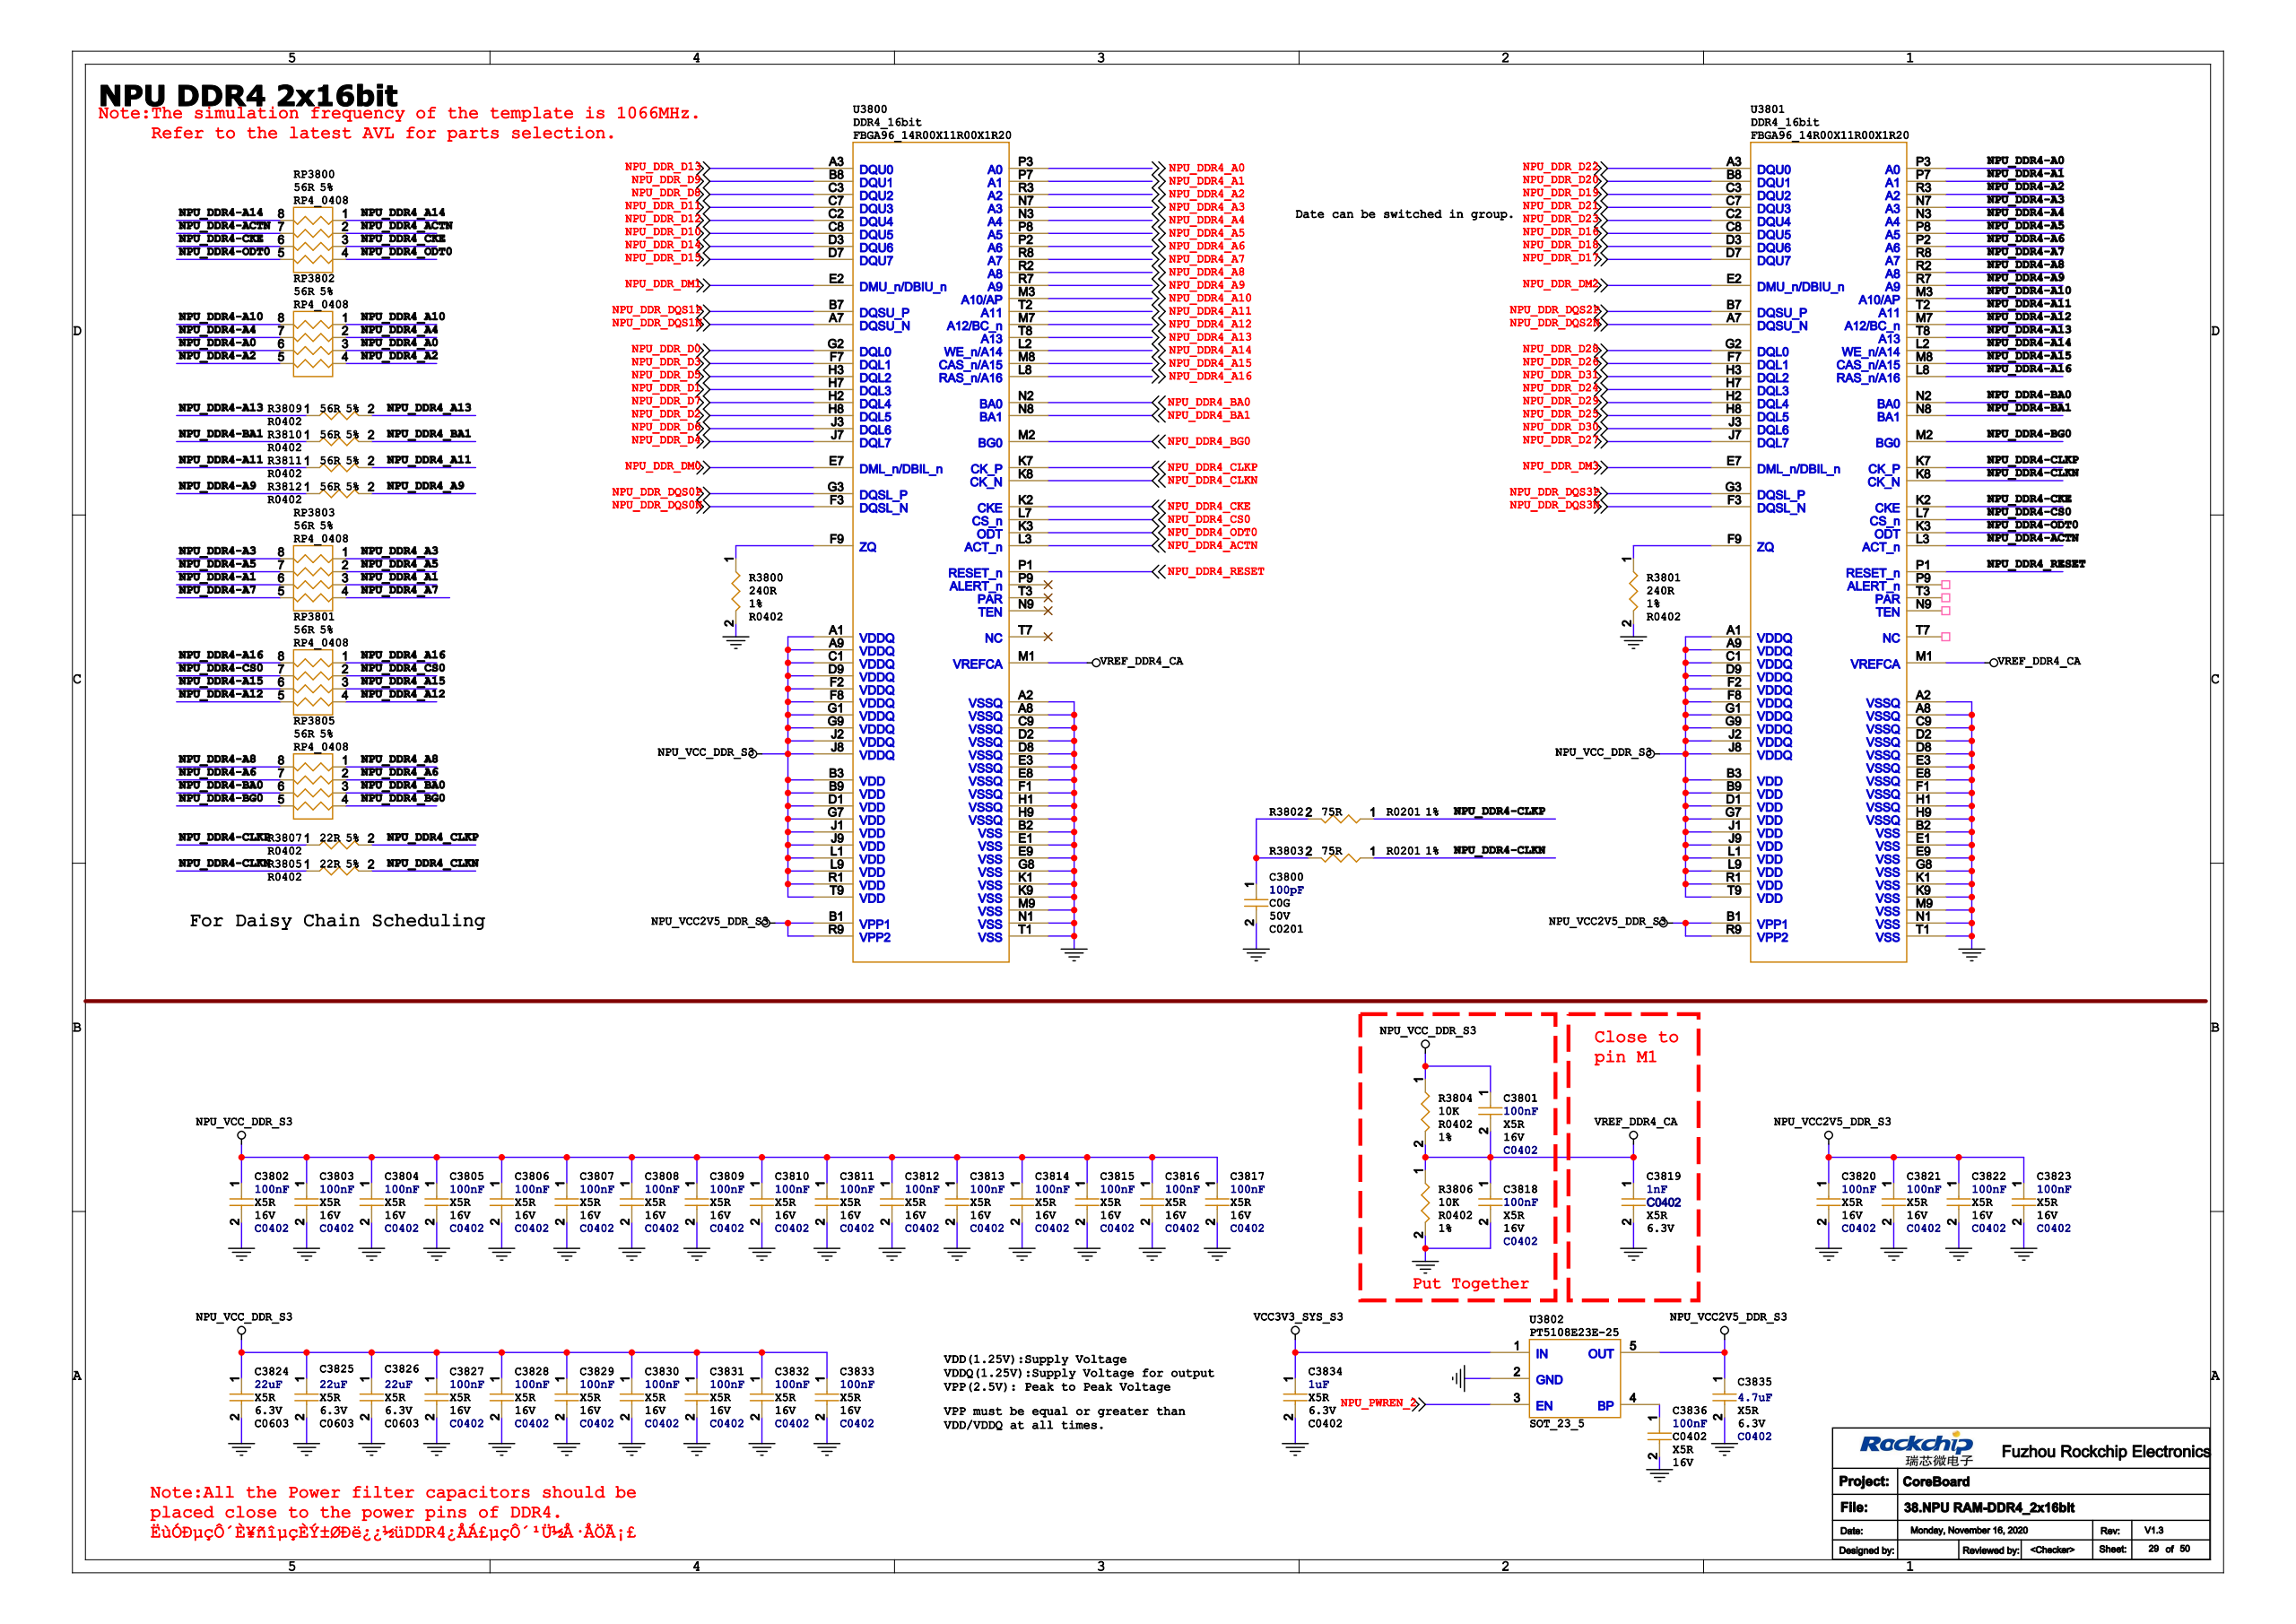Circuit board | Cadence Allegro | 749 parts | 717 nets | one sheet of the schematic
Parts on this sheet (reference | value | footprint):
C3800 | 100pF | C0201
C3801 | 100nF | C0402
C3802 | 100nF | C0402
C3803 | 100nF | C0402
C3804 | 100nF | C0402
C3805 | 100nF | C0402
C3806 | 100nF | C0402
C3807 | 100nF | C0402
C3808 | 100nF | C0402
C3809 | 100nF | C0402
C3810 | 100nF | C0402
C3811 | 100nF | C0402
C3812 | 100nF | C0402
C3813 | 100nF | C0402
C3814 | 100nF | C0402
C3815 | 100nF | C0402
C3816 | 100nF | C0402
C3817 | 100nF | C0402
C3818 | 100nF | C0402
C3819 | 1nF | C0402
C3820 | 100nF | C0402
C3821 | 100nF | C0402
C3822 | 100nF | C0402
C3823 | 100nF | C0402
C3824 | 22uF | C0603
C3825 | 22uF | C0603
C3826 | 22uF | C0603
C3827 | 100nF | C0402
C3828 | 100nF | C0402
C3829 | 100nF | C0402
C3830 | 100nF | C0402
C3831 | 100nF | C0402
C3832 | 100nF | C0402
C3833 | 100nF | C0402
C3834 | 1uF | C0402
C3835 | 4.7uF | C0402
C3836 | 100nF | C0402
R3800 | 240R | R0402
R3801 | 240R | R0402
R3804 | 10K | R0402
R3805 | 22R | R0402
R3806 | 10K | R0402
R3807 | 22R | R0402
R3809 | 56R | R0402
R3810 | 56R | R0402
R3811 | 56R | R0402
R3812 | 56R | R0402
RP3800 | 56R | RP4_0408
RP3801 | 56R | RP4_0408
RP3802 | 56R | RP4_0408
RP3803 | 56R | RP4_0408
RP3805 | 56R | RP4_0408
U3800 | DDR4_16bit | FBGA96_14R00X11R00X1R20
U3801 | DDR4_16bit | FBGA96_14R00X11R00X1R20
U3802 | PT5108E23E-25 | SOT_23_5
Nets of these parts (net: part-pin ...):
GND: C3800-2 C3802-2 C3803-2 C3804-2 C3805-2 C3806-2 C3807-2 C3808-2 C3809-2 C3810-2 C3811-2 C3812-2 C3813-2 C3814-2 C3815-2 C3816-2 C3817-2 C3818-2 C3819-2 C3820-2 C3821-2 C3822-2 C3823-2 C3824-2 C3825-2 C3826-2 C3827-2 C3828-2 C3829-2 C3830-2 C3831-2 C3832-2 C3833-2 C3834-2 C3835-2 C3836-2 R3800-2 R3801-2 R3806-2 U3802-2 U3800-A2 U3800-A8 U3800-B2 U3800-C9 U3800-D2 U3800-D8 U3800-E1 U3800-E3 U3800-E8 U3800-E9 U3800-F1 U3800-G8 U3800-H1 U3800-H9 U3800-K1 U3800-K9 U3800-M9 U3800-N1 U3800-T1 U3801-A2 U3801-A8 U3801-B2 U3801-C9 U3801-D2 U3801-D8 U3801-E1 U3801-E3 U3801-E8 U3801-E9 U3801-F1 U3801-G8 U3801-H1 U3801-H9 U3801-K1 U3801-K9 U3801-M9 U3801-N1 U3801-T1
VCC3V3_SYS_S3: C3834-1 U3802-1
NPU_VCC_DDR_S3: C3801-1 C3802-1 C3803-1 C3804-1 C3805-1 C3806-1 C3807-1 C3808-1 C3809-1 C3810-1 C3811-1 C3812-1 C3813-1 C3814-1 C3815-1 C3816-1 C3817-1 C3824-1 C3825-1 C3826-1 C3827-1 C3828-1 C3829-1 C3830-1 C3831-1 C3832-1 C3833-1 R3804-1 U3800-A1 U3800-A9 U3800-B3 U3800-B9 U3800-C1 U3800-D1 U3800-D9 U3800-F2 U3800-F8 U3800-G1 U3800-G7 U3800-G9 U3800-J1 U3800-J2 U3800-J8 U3800-J9 U3800-L1 U3800-L9 U3800-R1 U3800-T9 U3801-A1 U3801-A9 U3801-B3 U3801-B9 U3801-C1 U3801-D1 U3801-D9 U3801-F2 U3801-F8 U3801-G1 U3801-G7 U3801-G9 U3801-J1 U3801-J2 U3801-J8 U3801-J9 U3801-L1 U3801-L9 U3801-R1 U3801-T9
NPU_PWREN_2: U3802-3
NPU_DDR3_A0: RP3802-1 U3800-M3
NPU_DDR3_A12: R3810-2 U3800-N8
NPU_DDR3_A7: R3811-2 U3800-T2
NPU_DDR3_A8: R3809-2 U3800-T8
NPU_DDR3_BA0: RP3805-4 U3800-M2
NPU_DDR3_BA1: RP3801-3 U3800-M8
NPU_DDR3_BA2: RP3805-3 U3800-N2
NPU_DDR3_CASB: RP3801-4 U3800-M7
NPU_DDR3_CSB0: RP3800-2 U3800-L3
NPU_DDR3_ODT0: RP3800-1 U3800-L2
NPU_DDR3_RASB: RP3801-1 U3800-L8
NPU_DDR_DM0: U3800-E7
NPU_DDR_DM1: U3800-E2
NPU_DDR_DM2: U3801-E2
NPU_DDR_DM3: U3801-E7
NPU_DDR_D0: U3800-G2
NPU_DDR_D1: U3800-H7
NPU_DDR_D10: U3800-C8
NPU_DDR_D11: U3800-C7
NPU_DDR_D12: U3800-C2
NPU_DDR_D13: U3800-A3
NPU_DDR_D14: U3800-D3
NPU_DDR_D15: U3800-D7
NPU_DDR_D16: U3801-C8
NPU_DDR_D17: U3801-D7
NPU_DDR_D18: U3801-D3
NPU_DDR_D19: U3801-C3
NPU_DDR_D2: U3800-H8
NPU_DDR_D20: U3801-B8
NPU_DDR_D21: U3801-C7
NPU_DDR_D22: U3801-A3
NPU_DDR_D23: U3801-C2
NPU_DDR_D24: U3801-H7
NPU_DDR_D25: U3801-H8
NPU_DDR_D26: U3801-F7
NPU_DDR_D27: U3801-J7
NPU_DDR_D28: U3801-G2
NPU_DDR_D29: U3801-H2
NPU_DDR_D3: U3800-F7
NPU_DDR_D30: U3801-J3
NPU_DDR_D31: U3801-H3
NPU_DDR_D4: U3800-J7
NPU_DDR_D5: U3800-H3
NPU_DDR_D6: U3800-J3
NPU_DDR_D7: U3800-H2
NPU_DDR_D8: U3800-C3
NPU_DDR_D9: U3800-B8
NPU_DDR_DQS0N: U3800-F3
NPU_DDR_DQS0P: U3800-G3
NPU_DDR_DQS1N: U3800-A7
NPU_DDR_DQS1P: U3800-B7
NPU_DDR_DQS2N: U3801-A7
NPU_DDR_DQS2P: U3801-B7
NPU_DDR_DQS3N: U3801-F3
NPU_DDR_DQS3P: U3801-G3
NPU_DDR4_A0: RP3802-3 U3800-P3
NPU_DDR4_A1: RP3803-3 U3800-P7
NPU_DDR4_A2: RP3802-4 U3800-R3
NPU_DDR4_A3: RP3803-1 U3800-N7
NPU_DDR4_A4: RP3802-2 U3800-N3
NPU_DDR4_A5: RP3803-2 U3800-P8
NPU_DDR4_A6: RP3805-2 U3800-P2
NPU_DDR4_A7: RP3803-4 U3800-R8
NPU_DDR4_A8: RP3805-1 U3800-R2
NPU_DDR4_A9: R3812-2 U3800-R7
NPU_DDR4_CKE: RP3800-3 U3800-K2
NPU_DDR4_CLKP: R3807-2 U3800-K7
NPU_DDR4_CLKN: R3805-2 U3800-K8
NPU_DDR4_CS0: RP3801-2 U3800-L7
NPU_DDR4_ODT0: RP3800-4 U3800-K3
NPU_VCC2V5_DDR_S3: C3820-1 C3821-1 C3822-1 C3823-1 C3835-1 U3802-5 U3800-B1 U3800-R9 U3801-B1 U3801-R9
VREF_DDR4_CA: C3801-2 C3818-1 C3819-1 R3804-2 R3806-1 U3800-M1 U3801-M1
N77770852: R3800-1 U3800-F9
NPU_DDR4-A0: RP3802-6 U3801-P3
NPU_DDR4-A1: RP3803-6 U3801-P7
NPU_DDR4-A10: RP3802-8 U3801-M3
NPU_DDR4-A11: R3811-1 U3801-T2
NPU_DDR4-A12: RP3801-5 U3801-M7
NPU_DDR4-A13: R3809-1 U3801-T8
NPU_DDR4-A2: RP3802-5 U3801-R3
NPU_DDR4-A3: RP3803-8 U3801-N7
NPU_DDR4-A4: RP3802-7 U3801-N3
NPU_DDR4-A5: RP3803-7 U3801-P8
NPU_DDR4-A6: RP3805-7 U3801-P2
NPU_DDR4-A7: RP3803-5 U3801-R8
NPU_DDR4-A8: RP3805-8 U3801-R2
NPU_DDR4-A9: R3812-1 U3801-R7
NPU_DDR4-ACTN: RP3800-7 U3801-L3
NPU_DDR4-BA0: RP3805-6 U3801-N2
NPU_DDR4-BA1: R3810-1 U3801-N8
NPU_DDR4-BG0: RP3805-5 U3801-M2
NPU_DDR4-A15: RP3801-6 U3801-M8
NPU_DDR4-CKE: RP3800-6 U3801-K2
NPU_DDR4-CLKN: R3805-1 U3801-K8
NPU_DDR4-CLKP: R3807-1 U3801-K7
NPU_DDR4-CS0: RP3801-7 U3801-L7
NPU_DDR4-ODT0: RP3800-5 U3801-K3
NPU_DDR4-A16: RP3801-8 U3801-L8
NPU_DDR4-A14: RP3800-8 U3801-L2
N77770862: R3801-1 U3801-F9
N77772303: C3800-1
N83518949: C3836-1 U3802-4